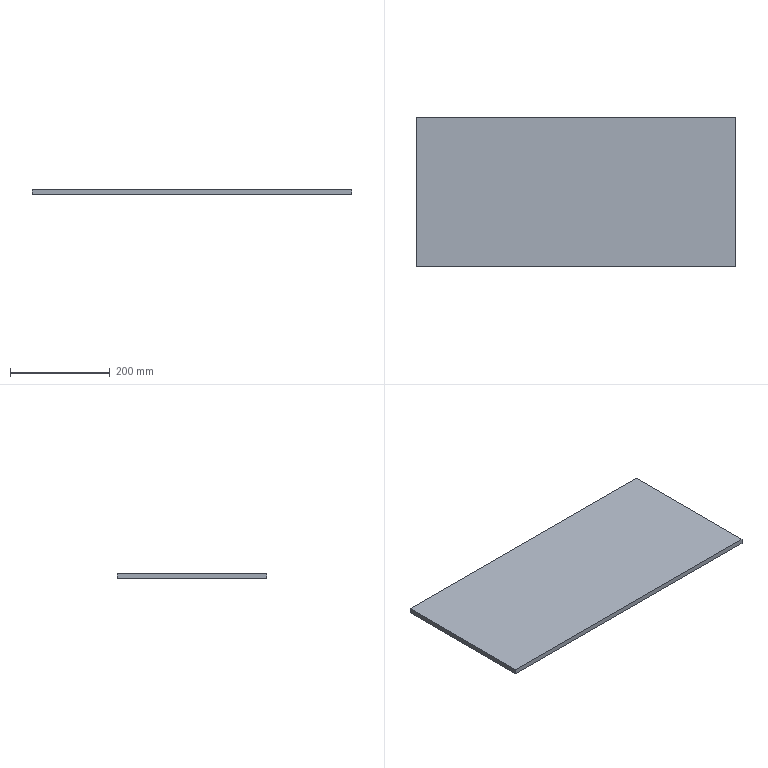Part | SolidWorks | features Extrusion 1 | 1 solid | 6 faces | box 640 x 300 x 10 mm | volume 1920000 mm3 | plane 6
STEP:
#1=CARTESIAN_POINT('',(0.,300.,0.));
#2=VERTEX_POINT('',#1);
#3=CARTESIAN_POINT('',(0.,0.,0.));
#4=VERTEX_POINT('',#3);
#5=CARTESIAN_POINT('',(0.,0.,0.));
#6=DIRECTION('',(0.,-1.,0.));
#7=VECTOR('',#6,1000.);
#8=LINE('',#5,#7);
#9=EDGE_CURVE('',#2,#4,#8,.T.);
#10=ORIENTED_EDGE('',*,*,#9,.T.);
#11=CARTESIAN_POINT('',(0.,0.,10.));
#12=VERTEX_POINT('',#11);
#13=CARTESIAN_POINT('',(0.,0.,10.));
#14=DIRECTION('',(0.,0.,-1.));
#15=VECTOR('',#14,1000.);
#16=LINE('',#13,#15);
#17=EDGE_CURVE('',#12,#4,#16,.T.);
#18=ORIENTED_EDGE('',*,*,#17,.F.);
#19=CARTESIAN_POINT('',(0.,300.,10.));
#20=VERTEX_POINT('',#19);
#21=CARTESIAN_POINT('',(0.,0.,10.));
#22=DIRECTION('',(0.,-1.,0.));
#23=VECTOR('',#22,1000.);
#24=LINE('',#21,#23);
#25=EDGE_CURVE('',#20,#12,#24,.T.);
#26=ORIENTED_EDGE('',*,*,#25,.F.);
#27=CARTESIAN_POINT('',(0.,300.,10.));
#28=DIRECTION('',(0.,0.,-1.));
#29=VECTOR('',#28,1000.);
#30=LINE('',#27,#29);
#31=EDGE_CURVE('',#20,#2,#30,.T.);
#32=ORIENTED_EDGE('',*,*,#31,.T.);
#33=EDGE_LOOP('',(#10,#18,#26,#32));
#34=FACE_OUTER_BOUND('',#33,.T.);
#35=CARTESIAN_POINT('',(0.,0.,10.));
#36=DIRECTION('',(1.,0.,0.));
#37=DIRECTION('',(0.,1.,0.));
#38=AXIS2_PLACEMENT_3D('',#35,#36,#37);
#39=PLANE('',#38);
#40=ADVANCED_FACE('',(#34),#39,.F.);
#41=CARTESIAN_POINT('',(640.,0.,0.));
#42=VERTEX_POINT('',#41);
#43=CARTESIAN_POINT('',(0.,0.,0.));
#44=DIRECTION('',(1.,0.,0.));
#45=VECTOR('',#44,1000.);
#46=LINE('',#43,#45);
#47=EDGE_CURVE('',#4,#42,#46,.T.);
#48=ORIENTED_EDGE('',*,*,#47,.T.);
#49=CARTESIAN_POINT('',(640.,0.,10.));
#50=VERTEX_POINT('',#49);
#51=CARTESIAN_POINT('',(640.,0.,10.));
#52=DIRECTION('',(0.,0.,-1.));
#53=VECTOR('',#52,1000.);
#54=LINE('',#51,#53);
#55=EDGE_CURVE('',#50,#42,#54,.T.);
#56=ORIENTED_EDGE('',*,*,#55,.F.);
#57=CARTESIAN_POINT('',(0.,0.,10.));
#58=DIRECTION('',(1.,0.,0.));
#59=VECTOR('',#58,1000.);
#60=LINE('',#57,#59);
#61=EDGE_CURVE('',#12,#50,#60,.T.);
#62=ORIENTED_EDGE('',*,*,#61,.F.);
#63=ORIENTED_EDGE('',*,*,#17,.T.);
#64=EDGE_LOOP('',(#48,#56,#62,#63));
#65=FACE_OUTER_BOUND('',#64,.T.);
#66=CARTESIAN_POINT('',(0.,0.,10.));
#67=DIRECTION('',(0.,1.,0.));
#68=DIRECTION('',(0.,0.,1.));
#69=AXIS2_PLACEMENT_3D('',#66,#67,#68);
#70=PLANE('',#69);
#71=ADVANCED_FACE('',(#65),#70,.F.);
#72=CARTESIAN_POINT('',(640.,300.,0.));
#73=VERTEX_POINT('',#72);
#74=CARTESIAN_POINT('',(640.,0.,0.));
#75=DIRECTION('',(0.,1.,0.));
#76=VECTOR('',#75,1000.);
#77=LINE('',#74,#76);
#78=EDGE_CURVE('',#42,#73,#77,.T.);
#79=ORIENTED_EDGE('',*,*,#78,.T.);
#80=CARTESIAN_POINT('',(640.,300.,10.));
#81=VERTEX_POINT('',#80);
#82=CARTESIAN_POINT('',(640.,300.,10.));
#83=DIRECTION('',(0.,0.,-1.));
#84=VECTOR('',#83,1000.);
#85=LINE('',#82,#84);
#86=EDGE_CURVE('',#81,#73,#85,.T.);
#87=ORIENTED_EDGE('',*,*,#86,.F.);
#88=CARTESIAN_POINT('',(640.,0.,10.));
#89=DIRECTION('',(0.,1.,0.));
#90=VECTOR('',#89,1000.);
#91=LINE('',#88,#90);
#92=EDGE_CURVE('',#50,#81,#91,.T.);
#93=ORIENTED_EDGE('',*,*,#92,.F.);
#94=ORIENTED_EDGE('',*,*,#55,.T.);
#95=EDGE_LOOP('',(#79,#87,#93,#94));
#96=FACE_OUTER_BOUND('',#95,.T.);
#97=CARTESIAN_POINT('',(640.,0.,10.));
#98=DIRECTION('',(-1.,0.,0.));
#99=DIRECTION('',(0.,0.,1.));
#100=AXIS2_PLACEMENT_3D('',#97,#98,#99);
#101=PLANE('',#100);
#102=ADVANCED_FACE('',(#96),#101,.F.);
#103=CARTESIAN_POINT('',(0.,300.,0.));
#104=DIRECTION('',(-1.,0.,0.));
#105=VECTOR('',#104,1000.);
#106=LINE('',#103,#105);
#107=EDGE_CURVE('',#73,#2,#106,.T.);
#108=ORIENTED_EDGE('',*,*,#107,.T.);
#109=ORIENTED_EDGE('',*,*,#31,.F.);
#110=CARTESIAN_POINT('',(0.,300.,10.));
#111=DIRECTION('',(-1.,0.,0.));
#112=VECTOR('',#111,1000.);
#113=LINE('',#110,#112);
#114=EDGE_CURVE('',#81,#20,#113,.T.);
#115=ORIENTED_EDGE('',*,*,#114,.F.);
#116=ORIENTED_EDGE('',*,*,#86,.T.);
#117=EDGE_LOOP('',(#108,#109,#115,#116));
#118=FACE_OUTER_BOUND('',#117,.T.);
#119=CARTESIAN_POINT('',(0.,300.,10.));
#120=DIRECTION('',(0.,-1.,0.));
#121=DIRECTION('',(0.,0.,-1.));
#122=AXIS2_PLACEMENT_3D('',#119,#120,#121);
#123=PLANE('',#122);
#124=ADVANCED_FACE('',(#118),#123,.F.);
#125=ORIENTED_EDGE('',*,*,#25,.T.);
#126=ORIENTED_EDGE('',*,*,#61,.T.);
#127=ORIENTED_EDGE('',*,*,#92,.T.);
#128=ORIENTED_EDGE('',*,*,#114,.T.);
#129=EDGE_LOOP('',(#125,#126,#127,#128));
#130=FACE_OUTER_BOUND('',#129,.T.);
#131=CARTESIAN_POINT('',(0.,0.,10.));
#132=DIRECTION('',(0.,0.,-1.));
#133=DIRECTION('',(-1.,0.,0.));
#134=AXIS2_PLACEMENT_3D('',#131,#132,#133);
#135=PLANE('',#134);
#136=ADVANCED_FACE('',(#130),#135,.F.);
#137=ORIENTED_EDGE('',*,*,#9,.F.);
#138=ORIENTED_EDGE('',*,*,#107,.F.);
#139=ORIENTED_EDGE('',*,*,#78,.F.);
#140=ORIENTED_EDGE('',*,*,#47,.F.);
#141=EDGE_LOOP('',(#137,#138,#139,#140));
#142=FACE_OUTER_BOUND('',#141,.T.);
#143=CARTESIAN_POINT('',(0.,0.,0.));
#144=DIRECTION('',(0.,0.,-1.));
#145=DIRECTION('',(-1.,0.,0.));
#146=AXIS2_PLACEMENT_3D('',#143,#144,#145);
#147=PLANE('',#146);
#148=ADVANCED_FACE('',(#142),#147,.T.);
#149=CLOSED_SHELL('',(#40,#71,#102,#124,#136,#148));
#150=MANIFOLD_SOLID_BREP('',#149);
#151=CARTESIAN_POINT('',(0.,0.,0.));
#152=DIRECTION('',(0.,0.,1.));
#153=DIRECTION('',(1.,0.,0.));
#154=AXIS2_PLACEMENT_3D('',#151,#152,#153);
#155=(LENGTH_UNIT()NAMED_UNIT(*)SI_UNIT(.MILLI.,.METRE.));
#156=UNCERTAINTY_MEASURE_WITH_UNIT(LENGTH_MEASURE(0.00001),#155,'','');
#157=(NAMED_UNIT(*)PLANE_ANGLE_UNIT()SI_UNIT($,.RADIAN.));
#158=(NAMED_UNIT(*)SI_UNIT($,.STERADIAN.)SOLID_ANGLE_UNIT());
#159=(GEOMETRIC_REPRESENTATION_CONTEXT(3)GLOBAL_UNCERTAINTY_ASSIGNED_CONTEXT((#156))GLOBAL_UNIT_ASSIGNED_CONTEXT((#155,#157,#158))REPRESENTATION_CONTEXT('',''));
#160=ADVANCED_BREP_SHAPE_REPRESENTATION('',(#150,#154),#159);